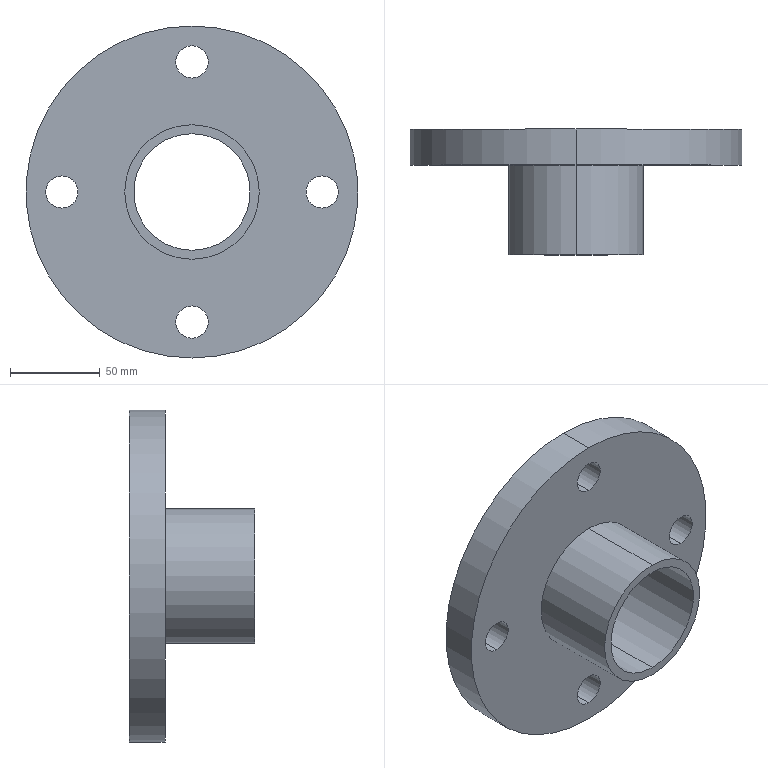Part | SolidWorks | features ICE 3, Extrusion 1 | 1 solid | 17 faces | box 185 x 70 x 185 mm | volume 505859 mm3 | cylinder 14 | plane 3 | commonest cylinder face diameters 18 x8 65 x2 75 x2 185 x2
STEP:
#1=CARTESIAN_POINT('',(0.,70.,63.5));
#2=VERTEX_POINT('',#1);
#3=CARTESIAN_POINT('',(0.,70.,81.5));
#4=VERTEX_POINT('',#3);
#5=CARTESIAN_POINT('',(0.,70.,72.5));
#6=DIRECTION('',(0.,1.,0.));
#7=DIRECTION('',(0.,0.,1.));
#8=AXIS2_PLACEMENT_3D('',#5,#6,#7);
#9=CIRCLE('',#8,9.);
#10=EDGE_CURVE('',#2,#4,#9,.T.);
#11=ORIENTED_EDGE('',*,*,#10,.T.);
#12=CARTESIAN_POINT('',(0.,50.,81.5));
#13=VERTEX_POINT('',#12);
#14=CARTESIAN_POINT('',(0.,70.,81.5));
#15=DIRECTION('',(0.,-1.,0.));
#16=VECTOR('',#15,1000.);
#17=LINE('',#14,#16);
#18=EDGE_CURVE('',#4,#13,#17,.T.);
#19=ORIENTED_EDGE('',*,*,#18,.T.);
#20=CARTESIAN_POINT('',(0.,50.,63.5));
#21=VERTEX_POINT('',#20);
#22=CARTESIAN_POINT('',(0.,50.,72.5));
#23=DIRECTION('',(0.,1.,0.));
#24=DIRECTION('',(0.,0.,1.));
#25=AXIS2_PLACEMENT_3D('',#22,#23,#24);
#26=CIRCLE('',#25,9.);
#27=EDGE_CURVE('',#21,#13,#26,.T.);
#28=ORIENTED_EDGE('',*,*,#27,.F.);
#29=CARTESIAN_POINT('',(0.,70.,63.5));
#30=DIRECTION('',(0.,-1.,0.));
#31=VECTOR('',#30,1000.);
#32=LINE('',#29,#31);
#33=EDGE_CURVE('',#2,#21,#32,.T.);
#34=ORIENTED_EDGE('',*,*,#33,.F.);
#35=EDGE_LOOP('',(#11,#19,#28,#34));
#36=FACE_OUTER_BOUND('',#35,.T.);
#37=CARTESIAN_POINT('',(0.,70.,72.5));
#38=DIRECTION('',(0.,-1.,0.));
#39=DIRECTION('',(0.,0.,-1.));
#40=AXIS2_PLACEMENT_3D('',#37,#38,#39);
#41=CYLINDRICAL_SURFACE('',#40,9.);
#42=ADVANCED_FACE('',(#36),#41,.F.);
#43=CARTESIAN_POINT('',(72.5,70.,-9.));
#44=VERTEX_POINT('',#43);
#45=CARTESIAN_POINT('',(72.5,70.,9.));
#46=VERTEX_POINT('',#45);
#47=CARTESIAN_POINT('',(72.5,70.,0.));
#48=DIRECTION('',(0.,1.,0.));
#49=DIRECTION('',(0.,0.,1.));
#50=AXIS2_PLACEMENT_3D('',#47,#48,#49);
#51=CIRCLE('',#50,9.);
#52=EDGE_CURVE('',#44,#46,#51,.T.);
#53=ORIENTED_EDGE('',*,*,#52,.T.);
#54=CARTESIAN_POINT('',(72.5,50.,9.));
#55=VERTEX_POINT('',#54);
#56=CARTESIAN_POINT('',(72.5,70.,9.));
#57=DIRECTION('',(0.,-1.,0.));
#58=VECTOR('',#57,1000.);
#59=LINE('',#56,#58);
#60=EDGE_CURVE('',#46,#55,#59,.T.);
#61=ORIENTED_EDGE('',*,*,#60,.T.);
#62=CARTESIAN_POINT('',(72.5,50.,-9.));
#63=VERTEX_POINT('',#62);
#64=CARTESIAN_POINT('',(72.5,50.,0.));
#65=DIRECTION('',(0.,1.,0.));
#66=DIRECTION('',(0.,0.,1.));
#67=AXIS2_PLACEMENT_3D('',#64,#65,#66);
#68=CIRCLE('',#67,9.);
#69=EDGE_CURVE('',#63,#55,#68,.T.);
#70=ORIENTED_EDGE('',*,*,#69,.F.);
#71=CARTESIAN_POINT('',(72.5,70.,-9.));
#72=DIRECTION('',(0.,-1.,0.));
#73=VECTOR('',#72,1000.);
#74=LINE('',#71,#73);
#75=EDGE_CURVE('',#44,#63,#74,.T.);
#76=ORIENTED_EDGE('',*,*,#75,.F.);
#77=EDGE_LOOP('',(#53,#61,#70,#76));
#78=FACE_OUTER_BOUND('',#77,.T.);
#79=CARTESIAN_POINT('',(72.5,70.,0.));
#80=DIRECTION('',(0.,-1.,0.));
#81=DIRECTION('',(0.,0.,-1.));
#82=AXIS2_PLACEMENT_3D('',#79,#80,#81);
#83=CYLINDRICAL_SURFACE('',#82,9.);
#84=ADVANCED_FACE('',(#78),#83,.F.);
#85=CARTESIAN_POINT('',(0.,70.,-81.5));
#86=VERTEX_POINT('',#85);
#87=CARTESIAN_POINT('',(0.,70.,-63.5));
#88=VERTEX_POINT('',#87);
#89=CARTESIAN_POINT('',(0.,70.,-72.5));
#90=DIRECTION('',(0.,1.,0.));
#91=DIRECTION('',(0.,0.,1.));
#92=AXIS2_PLACEMENT_3D('',#89,#90,#91);
#93=CIRCLE('',#92,9.);
#94=EDGE_CURVE('',#86,#88,#93,.T.);
#95=ORIENTED_EDGE('',*,*,#94,.T.);
#96=CARTESIAN_POINT('',(0.,50.,-63.5));
#97=VERTEX_POINT('',#96);
#98=CARTESIAN_POINT('',(0.,70.,-63.5));
#99=DIRECTION('',(0.,-1.,0.));
#100=VECTOR('',#99,1000.);
#101=LINE('',#98,#100);
#102=EDGE_CURVE('',#88,#97,#101,.T.);
#103=ORIENTED_EDGE('',*,*,#102,.T.);
#104=CARTESIAN_POINT('',(0.,50.,-81.5));
#105=VERTEX_POINT('',#104);
#106=CARTESIAN_POINT('',(0.,50.,-72.5));
#107=DIRECTION('',(0.,1.,0.));
#108=DIRECTION('',(0.,0.,1.));
#109=AXIS2_PLACEMENT_3D('',#106,#107,#108);
#110=CIRCLE('',#109,9.);
#111=EDGE_CURVE('',#105,#97,#110,.T.);
#112=ORIENTED_EDGE('',*,*,#111,.F.);
#113=CARTESIAN_POINT('',(0.,70.,-81.5));
#114=DIRECTION('',(0.,-1.,0.));
#115=VECTOR('',#114,1000.);
#116=LINE('',#113,#115);
#117=EDGE_CURVE('',#86,#105,#116,.T.);
#118=ORIENTED_EDGE('',*,*,#117,.F.);
#119=EDGE_LOOP('',(#95,#103,#112,#118));
#120=FACE_OUTER_BOUND('',#119,.T.);
#121=CARTESIAN_POINT('',(0.,70.,-72.5));
#122=DIRECTION('',(0.,-1.,0.));
#123=DIRECTION('',(0.,0.,-1.));
#124=AXIS2_PLACEMENT_3D('',#121,#122,#123);
#125=CYLINDRICAL_SURFACE('',#124,9.);
#126=ADVANCED_FACE('',(#120),#125,.F.);
#127=CARTESIAN_POINT('',(-72.5,70.,-9.));
#128=VERTEX_POINT('',#127);
#129=CARTESIAN_POINT('',(-72.5,70.,9.));
#130=VERTEX_POINT('',#129);
#131=CARTESIAN_POINT('',(-72.5,70.,0.));
#132=DIRECTION('',(0.,1.,0.));
#133=DIRECTION('',(0.,0.,1.));
#134=AXIS2_PLACEMENT_3D('',#131,#132,#133);
#135=CIRCLE('',#134,9.);
#136=EDGE_CURVE('',#128,#130,#135,.T.);
#137=ORIENTED_EDGE('',*,*,#136,.T.);
#138=CARTESIAN_POINT('',(-72.5,50.,9.));
#139=VERTEX_POINT('',#138);
#140=CARTESIAN_POINT('',(-72.5,70.,9.));
#141=DIRECTION('',(0.,-1.,0.));
#142=VECTOR('',#141,1000.);
#143=LINE('',#140,#142);
#144=EDGE_CURVE('',#130,#139,#143,.T.);
#145=ORIENTED_EDGE('',*,*,#144,.T.);
#146=CARTESIAN_POINT('',(-72.5,50.,-9.));
#147=VERTEX_POINT('',#146);
#148=CARTESIAN_POINT('',(-72.5,50.,0.));
#149=DIRECTION('',(0.,1.,0.));
#150=DIRECTION('',(0.,0.,1.));
#151=AXIS2_PLACEMENT_3D('',#148,#149,#150);
#152=CIRCLE('',#151,9.);
#153=EDGE_CURVE('',#147,#139,#152,.T.);
#154=ORIENTED_EDGE('',*,*,#153,.F.);
#155=CARTESIAN_POINT('',(-72.5,70.,-9.));
#156=DIRECTION('',(0.,-1.,0.));
#157=VECTOR('',#156,1000.);
#158=LINE('',#155,#157);
#159=EDGE_CURVE('',#128,#147,#158,.T.);
#160=ORIENTED_EDGE('',*,*,#159,.F.);
#161=EDGE_LOOP('',(#137,#145,#154,#160));
#162=FACE_OUTER_BOUND('',#161,.T.);
#163=CARTESIAN_POINT('',(-72.5,70.,0.));
#164=DIRECTION('',(0.,-1.,0.));
#165=DIRECTION('',(0.,0.,-1.));
#166=AXIS2_PLACEMENT_3D('',#163,#164,#165);
#167=CYLINDRICAL_SURFACE('',#166,9.);
#168=ADVANCED_FACE('',(#162),#167,.F.);
#169=CARTESIAN_POINT('',(0.,70.,92.5));
#170=VERTEX_POINT('',#169);
#171=CARTESIAN_POINT('',(0.,70.,-92.5));
#172=VERTEX_POINT('',#171);
#173=CARTESIAN_POINT('',(0.,70.,0.));
#174=DIRECTION('',(0.,1.,0.));
#175=DIRECTION('',(0.,0.,1.));
#176=AXIS2_PLACEMENT_3D('',#173,#174,#175);
#177=CIRCLE('',#176,92.5);
#178=EDGE_CURVE('',#170,#172,#177,.T.);
#179=ORIENTED_EDGE('',*,*,#178,.F.);
#180=CARTESIAN_POINT('',(0.,50.,92.5));
#181=VERTEX_POINT('',#180);
#182=CARTESIAN_POINT('',(0.,70.,92.5));
#183=DIRECTION('',(0.,-1.,0.));
#184=VECTOR('',#183,1000.);
#185=LINE('',#182,#184);
#186=EDGE_CURVE('',#170,#181,#185,.T.);
#187=ORIENTED_EDGE('',*,*,#186,.T.);
#188=CARTESIAN_POINT('',(0.,50.,-92.5));
#189=VERTEX_POINT('',#188);
#190=CARTESIAN_POINT('',(0.,50.,0.));
#191=DIRECTION('',(0.,1.,0.));
#192=DIRECTION('',(0.,0.,1.));
#193=AXIS2_PLACEMENT_3D('',#190,#191,#192);
#194=CIRCLE('',#193,92.5);
#195=EDGE_CURVE('',#181,#189,#194,.T.);
#196=ORIENTED_EDGE('',*,*,#195,.T.);
#197=CARTESIAN_POINT('',(0.,70.,-92.5));
#198=DIRECTION('',(0.,-1.,0.));
#199=VECTOR('',#198,1000.);
#200=LINE('',#197,#199);
#201=EDGE_CURVE('',#172,#189,#200,.T.);
#202=ORIENTED_EDGE('',*,*,#201,.F.);
#203=EDGE_LOOP('',(#179,#187,#196,#202));
#204=FACE_OUTER_BOUND('',#203,.T.);
#205=CARTESIAN_POINT('',(0.,70.,0.));
#206=DIRECTION('',(0.,-1.,0.));
#207=DIRECTION('',(0.,0.,-1.));
#208=AXIS2_PLACEMENT_3D('',#205,#206,#207);
#209=CYLINDRICAL_SURFACE('',#208,92.5);
#210=ADVANCED_FACE('',(#204),#209,.T.);
#211=CARTESIAN_POINT('',(0.,70.,32.5));
#212=VERTEX_POINT('',#211);
#213=CARTESIAN_POINT('',(0.,70.,-32.5));
#214=VERTEX_POINT('',#213);
#215=CARTESIAN_POINT('',(0.,70.,0.));
#216=DIRECTION('',(0.,-1.,0.));
#217=DIRECTION('',(0.,0.,-1.));
#218=AXIS2_PLACEMENT_3D('',#215,#216,#217);
#219=CIRCLE('',#218,32.5);
#220=EDGE_CURVE('',#212,#214,#219,.T.);
#221=ORIENTED_EDGE('',*,*,#220,.F.);
#222=CARTESIAN_POINT('',(0.,0.,32.5));
#223=VERTEX_POINT('',#222);
#224=CARTESIAN_POINT('',(0.,50.,32.5));
#225=DIRECTION('',(0.,-1.,0.));
#226=VECTOR('',#225,1000.);
#227=LINE('',#224,#226);
#228=EDGE_CURVE('',#212,#223,#227,.T.);
#229=ORIENTED_EDGE('',*,*,#228,.T.);
#230=CARTESIAN_POINT('',(0.,0.,-32.5));
#231=VERTEX_POINT('',#230);
#232=CARTESIAN_POINT('',(0.,0.,0.));
#233=DIRECTION('',(0.,1.,0.));
#234=DIRECTION('',(0.,0.,1.));
#235=AXIS2_PLACEMENT_3D('',#232,#233,#234);
#236=CIRCLE('',#235,32.5);
#237=EDGE_CURVE('',#231,#223,#236,.T.);
#238=ORIENTED_EDGE('',*,*,#237,.F.);
#239=CARTESIAN_POINT('',(0.,50.,-32.5));
#240=DIRECTION('',(0.,-1.,0.));
#241=VECTOR('',#240,1000.);
#242=LINE('',#239,#241);
#243=EDGE_CURVE('',#214,#231,#242,.T.);
#244=ORIENTED_EDGE('',*,*,#243,.F.);
#245=EDGE_LOOP('',(#221,#229,#238,#244));
#246=FACE_OUTER_BOUND('',#245,.T.);
#247=CARTESIAN_POINT('',(0.,50.,0.));
#248=DIRECTION('',(0.,-1.,0.));
#249=DIRECTION('',(0.,0.,-1.));
#250=AXIS2_PLACEMENT_3D('',#247,#248,#249);
#251=CYLINDRICAL_SURFACE('',#250,32.5);
#252=ADVANCED_FACE('',(#246),#251,.F.);
#253=CARTESIAN_POINT('',(0.,50.,37.5));
#254=VERTEX_POINT('',#253);
#255=CARTESIAN_POINT('',(0.,50.,-37.5));
#256=VERTEX_POINT('',#255);
#257=CARTESIAN_POINT('',(0.,50.,0.));
#258=DIRECTION('',(0.,1.,0.));
#259=DIRECTION('',(0.,0.,1.));
#260=AXIS2_PLACEMENT_3D('',#257,#258,#259);
#261=CIRCLE('',#260,37.5);
#262=EDGE_CURVE('',#254,#256,#261,.T.);
#263=ORIENTED_EDGE('',*,*,#262,.F.);
#264=CARTESIAN_POINT('',(0.,0.,37.5));
#265=VERTEX_POINT('',#264);
#266=CARTESIAN_POINT('',(0.,50.,37.5));
#267=DIRECTION('',(0.,-1.,0.));
#268=VECTOR('',#267,1000.);
#269=LINE('',#266,#268);
#270=EDGE_CURVE('',#254,#265,#269,.T.);
#271=ORIENTED_EDGE('',*,*,#270,.T.);
#272=CARTESIAN_POINT('',(0.,0.,-37.5));
#273=VERTEX_POINT('',#272);
#274=CARTESIAN_POINT('',(0.,0.,0.));
#275=DIRECTION('',(0.,1.,0.));
#276=DIRECTION('',(0.,0.,1.));
#277=AXIS2_PLACEMENT_3D('',#274,#275,#276);
#278=CIRCLE('',#277,37.5);
#279=EDGE_CURVE('',#265,#273,#278,.T.);
#280=ORIENTED_EDGE('',*,*,#279,.T.);
#281=CARTESIAN_POINT('',(0.,50.,-37.5));
#282=DIRECTION('',(0.,-1.,0.));
#283=VECTOR('',#282,1000.);
#284=LINE('',#281,#283);
#285=EDGE_CURVE('',#256,#273,#284,.T.);
#286=ORIENTED_EDGE('',*,*,#285,.F.);
#287=EDGE_LOOP('',(#263,#271,#280,#286));
#288=FACE_OUTER_BOUND('',#287,.T.);
#289=CARTESIAN_POINT('',(0.,50.,0.));
#290=DIRECTION('',(0.,-1.,0.));
#291=DIRECTION('',(0.,0.,-1.));
#292=AXIS2_PLACEMENT_3D('',#289,#290,#291);
#293=CYLINDRICAL_SURFACE('',#292,37.5);
#294=ADVANCED_FACE('',(#288),#293,.T.);
#295=ORIENTED_EDGE('',*,*,#270,.F.);
#296=CARTESIAN_POINT('',(0.,50.,0.));
#297=DIRECTION('',(0.,1.,0.));
#298=DIRECTION('',(0.,0.,1.));
#299=AXIS2_PLACEMENT_3D('',#296,#297,#298);
#300=CIRCLE('',#299,37.5);
#301=EDGE_CURVE('',#256,#254,#300,.T.);
#302=ORIENTED_EDGE('',*,*,#301,.F.);
#303=ORIENTED_EDGE('',*,*,#285,.T.);
#304=CARTESIAN_POINT('',(0.,0.,0.));
#305=DIRECTION('',(0.,1.,0.));
#306=DIRECTION('',(0.,0.,1.));
#307=AXIS2_PLACEMENT_3D('',#304,#305,#306);
#308=CIRCLE('',#307,37.5);
#309=EDGE_CURVE('',#273,#265,#308,.T.);
#310=ORIENTED_EDGE('',*,*,#309,.T.);
#311=EDGE_LOOP('',(#295,#302,#303,#310));
#312=FACE_OUTER_BOUND('',#311,.T.);
#313=CARTESIAN_POINT('',(0.,50.,0.));
#314=DIRECTION('',(0.,-1.,0.));
#315=DIRECTION('',(0.,0.,-1.));
#316=AXIS2_PLACEMENT_3D('',#313,#314,#315);
#317=CYLINDRICAL_SURFACE('',#316,37.5);
#318=ADVANCED_FACE('',(#312),#317,.T.);
#319=ORIENTED_EDGE('',*,*,#309,.F.);
#320=ORIENTED_EDGE('',*,*,#279,.F.);
#321=EDGE_LOOP('',(#319,#320));
#322=FACE_OUTER_BOUND('',#321,.T.);
#323=ORIENTED_EDGE('',*,*,#237,.T.);
#324=CARTESIAN_POINT('',(0.,0.,0.));
#325=DIRECTION('',(0.,1.,0.));
#326=DIRECTION('',(0.,0.,1.));
#327=AXIS2_PLACEMENT_3D('',#324,#325,#326);
#328=CIRCLE('',#327,32.5);
#329=EDGE_CURVE('',#223,#231,#328,.T.);
#330=ORIENTED_EDGE('',*,*,#329,.T.);
#331=EDGE_LOOP('',(#323,#330));
#332=FACE_BOUND('',#331,.T.);
#333=CARTESIAN_POINT('',(0.,0.,0.));
#334=DIRECTION('',(0.,1.,0.));
#335=DIRECTION('',(0.,0.,1.));
#336=AXIS2_PLACEMENT_3D('',#333,#334,#335);
#337=PLANE('',#336);
#338=ADVANCED_FACE('',(#322,#332),#337,.F.);
#339=ORIENTED_EDGE('',*,*,#228,.F.);
#340=CARTESIAN_POINT('',(0.,70.,0.));
#341=DIRECTION('',(0.,-1.,0.));
#342=DIRECTION('',(0.,0.,-1.));
#343=AXIS2_PLACEMENT_3D('',#340,#341,#342);
#344=CIRCLE('',#343,32.5);
#345=EDGE_CURVE('',#214,#212,#344,.T.);
#346=ORIENTED_EDGE('',*,*,#345,.F.);
#347=ORIENTED_EDGE('',*,*,#243,.T.);
#348=ORIENTED_EDGE('',*,*,#329,.F.);
#349=EDGE_LOOP('',(#339,#346,#347,#348));
#350=FACE_OUTER_BOUND('',#349,.T.);
#351=CARTESIAN_POINT('',(0.,50.,0.));
#352=DIRECTION('',(0.,-1.,0.));
#353=DIRECTION('',(0.,0.,-1.));
#354=AXIS2_PLACEMENT_3D('',#351,#352,#353);
#355=CYLINDRICAL_SURFACE('',#354,32.5);
#356=ADVANCED_FACE('',(#350),#355,.F.);
#357=CARTESIAN_POINT('',(0.,50.,0.));
#358=DIRECTION('',(0.,1.,0.));
#359=DIRECTION('',(0.,0.,1.));
#360=AXIS2_PLACEMENT_3D('',#357,#358,#359);
#361=CIRCLE('',#360,92.5);
#362=EDGE_CURVE('',#189,#181,#361,.T.);
#363=ORIENTED_EDGE('',*,*,#362,.F.);
#364=ORIENTED_EDGE('',*,*,#195,.F.);
#365=EDGE_LOOP('',(#363,#364));
#366=FACE_OUTER_BOUND('',#365,.T.);
#367=ORIENTED_EDGE('',*,*,#301,.T.);
#368=ORIENTED_EDGE('',*,*,#262,.T.);
#369=EDGE_LOOP('',(#367,#368));
#370=FACE_BOUND('',#369,.T.);
#371=ORIENTED_EDGE('',*,*,#153,.T.);
#372=CARTESIAN_POINT('',(-72.5,50.,0.));
#373=DIRECTION('',(0.,1.,0.));
#374=DIRECTION('',(0.,0.,1.));
#375=AXIS2_PLACEMENT_3D('',#372,#373,#374);
#376=CIRCLE('',#375,9.);
#377=EDGE_CURVE('',#139,#147,#376,.T.);
#378=ORIENTED_EDGE('',*,*,#377,.T.);
#379=EDGE_LOOP('',(#371,#378));
#380=FACE_BOUND('',#379,.T.);
#381=ORIENTED_EDGE('',*,*,#111,.T.);
#382=CARTESIAN_POINT('',(0.,50.,-72.5));
#383=DIRECTION('',(0.,1.,0.));
#384=DIRECTION('',(0.,0.,1.));
#385=AXIS2_PLACEMENT_3D('',#382,#383,#384);
#386=CIRCLE('',#385,9.);
#387=EDGE_CURVE('',#97,#105,#386,.T.);
#388=ORIENTED_EDGE('',*,*,#387,.T.);
#389=EDGE_LOOP('',(#381,#388));
#390=FACE_BOUND('',#389,.T.);
#391=ORIENTED_EDGE('',*,*,#69,.T.);
#392=CARTESIAN_POINT('',(72.5,50.,0.));
#393=DIRECTION('',(0.,1.,0.));
#394=DIRECTION('',(0.,0.,1.));
#395=AXIS2_PLACEMENT_3D('',#392,#393,#394);
#396=CIRCLE('',#395,9.);
#397=EDGE_CURVE('',#55,#63,#396,.T.);
#398=ORIENTED_EDGE('',*,*,#397,.T.);
#399=EDGE_LOOP('',(#391,#398));
#400=FACE_BOUND('',#399,.T.);
#401=ORIENTED_EDGE('',*,*,#27,.T.);
#402=CARTESIAN_POINT('',(0.,50.,72.5));
#403=DIRECTION('',(0.,1.,0.));
#404=DIRECTION('',(0.,0.,1.));
#405=AXIS2_PLACEMENT_3D('',#402,#403,#404);
#406=CIRCLE('',#405,9.);
#407=EDGE_CURVE('',#13,#21,#406,.T.);
#408=ORIENTED_EDGE('',*,*,#407,.T.);
#409=EDGE_LOOP('',(#401,#408));
#410=FACE_BOUND('',#409,.T.);
#411=CARTESIAN_POINT('',(0.,50.,0.));
#412=DIRECTION('',(0.,1.,0.));
#413=DIRECTION('',(0.,0.,1.));
#414=AXIS2_PLACEMENT_3D('',#411,#412,#413);
#415=PLANE('',#414);
#416=ADVANCED_FACE('',(#366,#370,#380,#390,#400,#410),#415,.F.);
#417=ORIENTED_EDGE('',*,*,#186,.F.);
#418=CARTESIAN_POINT('',(0.,70.,0.));
#419=DIRECTION('',(0.,1.,0.));
#420=DIRECTION('',(0.,0.,1.));
#421=AXIS2_PLACEMENT_3D('',#418,#419,#420);
#422=CIRCLE('',#421,92.5);
#423=EDGE_CURVE('',#172,#170,#422,.T.);
#424=ORIENTED_EDGE('',*,*,#423,.F.);
#425=ORIENTED_EDGE('',*,*,#201,.T.);
#426=ORIENTED_EDGE('',*,*,#362,.T.);
#427=EDGE_LOOP('',(#417,#424,#425,#426));
#428=FACE_OUTER_BOUND('',#427,.T.);
#429=CARTESIAN_POINT('',(0.,70.,0.));
#430=DIRECTION('',(0.,-1.,0.));
#431=DIRECTION('',(0.,0.,-1.));
#432=AXIS2_PLACEMENT_3D('',#429,#430,#431);
#433=CYLINDRICAL_SURFACE('',#432,92.5);
#434=ADVANCED_FACE('',(#428),#433,.T.);
#435=ORIENTED_EDGE('',*,*,#144,.F.);
#436=CARTESIAN_POINT('',(-72.5,70.,0.));
#437=DIRECTION('',(0.,1.,0.));
#438=DIRECTION('',(0.,0.,1.));
#439=AXIS2_PLACEMENT_3D('',#436,#437,#438);
#440=CIRCLE('',#439,9.);
#441=EDGE_CURVE('',#130,#128,#440,.T.);
#442=ORIENTED_EDGE('',*,*,#441,.T.);
#443=ORIENTED_EDGE('',*,*,#159,.T.);
#444=ORIENTED_EDGE('',*,*,#377,.F.);
#445=EDGE_LOOP('',(#435,#442,#443,#444));
#446=FACE_OUTER_BOUND('',#445,.T.);
#447=CARTESIAN_POINT('',(-72.5,70.,0.));
#448=DIRECTION('',(0.,-1.,0.));
#449=DIRECTION('',(0.,0.,-1.));
#450=AXIS2_PLACEMENT_3D('',#447,#448,#449);
#451=CYLINDRICAL_SURFACE('',#450,9.);
#452=ADVANCED_FACE('',(#446),#451,.F.);
#453=ORIENTED_EDGE('',*,*,#102,.F.);
#454=CARTESIAN_POINT('',(0.,70.,-72.5));
#455=DIRECTION('',(0.,1.,0.));
#456=DIRECTION('',(0.,0.,1.));
#457=AXIS2_PLACEMENT_3D('',#454,#455,#456);
#458=CIRCLE('',#457,9.);
#459=EDGE_CURVE('',#88,#86,#458,.T.);
#460=ORIENTED_EDGE('',*,*,#459,.T.);
#461=ORIENTED_EDGE('',*,*,#117,.T.);
#462=ORIENTED_EDGE('',*,*,#387,.F.);
#463=EDGE_LOOP('',(#453,#460,#461,#462));
#464=FACE_OUTER_BOUND('',#463,.T.);
#465=CARTESIAN_POINT('',(0.,70.,-72.5));
#466=DIRECTION('',(0.,-1.,0.));
#467=DIRECTION('',(0.,0.,-1.));
#468=AXIS2_PLACEMENT_3D('',#465,#466,#467);
#469=CYLINDRICAL_SURFACE('',#468,9.);
#470=ADVANCED_FACE('',(#464),#469,.F.);
#471=ORIENTED_EDGE('',*,*,#60,.F.);
#472=CARTESIAN_POINT('',(72.5,70.,0.));
#473=DIRECTION('',(0.,1.,0.));
#474=DIRECTION('',(0.,0.,1.));
#475=AXIS2_PLACEMENT_3D('',#472,#473,#474);
#476=CIRCLE('',#475,9.);
#477=EDGE_CURVE('',#46,#44,#476,.T.);
#478=ORIENTED_EDGE('',*,*,#477,.T.);
#479=ORIENTED_EDGE('',*,*,#75,.T.);
#480=ORIENTED_EDGE('',*,*,#397,.F.);
#481=EDGE_LOOP('',(#471,#478,#479,#480));
#482=FACE_OUTER_BOUND('',#481,.T.);
#483=CARTESIAN_POINT('',(72.5,70.,0.));
#484=DIRECTION('',(0.,-1.,0.));
#485=DIRECTION('',(0.,0.,-1.));
#486=AXIS2_PLACEMENT_3D('',#483,#484,#485);
#487=CYLINDRICAL_SURFACE('',#486,9.);
#488=ADVANCED_FACE('',(#482),#487,.F.);
#489=ORIENTED_EDGE('',*,*,#18,.F.);
#490=CARTESIAN_POINT('',(0.,70.,72.5));
#491=DIRECTION('',(0.,1.,0.));
#492=DIRECTION('',(0.,0.,1.));
#493=AXIS2_PLACEMENT_3D('',#490,#491,#492);
#494=CIRCLE('',#493,9.);
#495=EDGE_CURVE('',#4,#2,#494,.T.);
#496=ORIENTED_EDGE('',*,*,#495,.T.);
#497=ORIENTED_EDGE('',*,*,#33,.T.);
#498=ORIENTED_EDGE('',*,*,#407,.F.);
#499=EDGE_LOOP('',(#489,#496,#497,#498));
#500=FACE_OUTER_BOUND('',#499,.T.);
#501=CARTESIAN_POINT('',(0.,70.,72.5));
#502=DIRECTION('',(0.,-1.,0.));
#503=DIRECTION('',(0.,0.,-1.));
#504=AXIS2_PLACEMENT_3D('',#501,#502,#503);
#505=CYLINDRICAL_SURFACE('',#504,9.);
#506=ADVANCED_FACE('',(#500),#505,.F.);
#507=ORIENTED_EDGE('',*,*,#345,.T.);
#508=ORIENTED_EDGE('',*,*,#220,.T.);
#509=EDGE_LOOP('',(#507,#508));
#510=FACE_BOUND('',#509,.T.);
#511=ORIENTED_EDGE('',*,*,#52,.F.);
#512=ORIENTED_EDGE('',*,*,#477,.F.);
#513=EDGE_LOOP('',(#511,#512));
#514=FACE_BOUND('',#513,.T.);
#515=ORIENTED_EDGE('',*,*,#136,.F.);
#516=ORIENTED_EDGE('',*,*,#441,.F.);
#517=EDGE_LOOP('',(#515,#516));
#518=FACE_BOUND('',#517,.T.);
#519=ORIENTED_EDGE('',*,*,#423,.T.);
#520=ORIENTED_EDGE('',*,*,#178,.T.);
#521=EDGE_LOOP('',(#519,#520));
#522=FACE_OUTER_BOUND('',#521,.T.);
#523=ORIENTED_EDGE('',*,*,#94,.F.);
#524=ORIENTED_EDGE('',*,*,#459,.F.);
#525=EDGE_LOOP('',(#523,#524));
#526=FACE_BOUND('',#525,.T.);
#527=ORIENTED_EDGE('',*,*,#10,.F.);
#528=ORIENTED_EDGE('',*,*,#495,.F.);
#529=EDGE_LOOP('',(#527,#528));
#530=FACE_BOUND('',#529,.T.);
#531=CARTESIAN_POINT('',(0.,70.,0.));
#532=DIRECTION('',(0.,1.,0.));
#533=DIRECTION('',(0.,0.,1.));
#534=AXIS2_PLACEMENT_3D('',#531,#532,#533);
#535=PLANE('',#534);
#536=ADVANCED_FACE('',(#510,#514,#518,#522,#526,#530),#535,.T.);
#537=CLOSED_SHELL('',(#42,#84,#126,#168,#210,#252,#294,#318,#338,#356,#416,#434,#452,#470,#488,#506,#536));
#538=MANIFOLD_SOLID_BREP('',#537);
#539=CARTESIAN_POINT('',(0.,0.,0.));
#540=DIRECTION('',(0.,0.,1.));
#541=DIRECTION('',(1.,0.,0.));
#542=AXIS2_PLACEMENT_3D('',#539,#540,#541);
#543=(LENGTH_UNIT()NAMED_UNIT(*)SI_UNIT(.MILLI.,.METRE.));
#544=UNCERTAINTY_MEASURE_WITH_UNIT(LENGTH_MEASURE(0.00001),#543,'','');
#545=(NAMED_UNIT(*)PLANE_ANGLE_UNIT()SI_UNIT($,.RADIAN.));
#546=(NAMED_UNIT(*)SI_UNIT($,.STERADIAN.)SOLID_ANGLE_UNIT());
#547=(GEOMETRIC_REPRESENTATION_CONTEXT(3)GLOBAL_UNCERTAINTY_ASSIGNED_CONTEXT((#544))GLOBAL_UNIT_ASSIGNED_CONTEXT((#543,#545,#546))REPRESENTATION_CONTEXT('',''));
#548=ADVANCED_BREP_SHAPE_REPRESENTATION('',(#538,#542),#547);